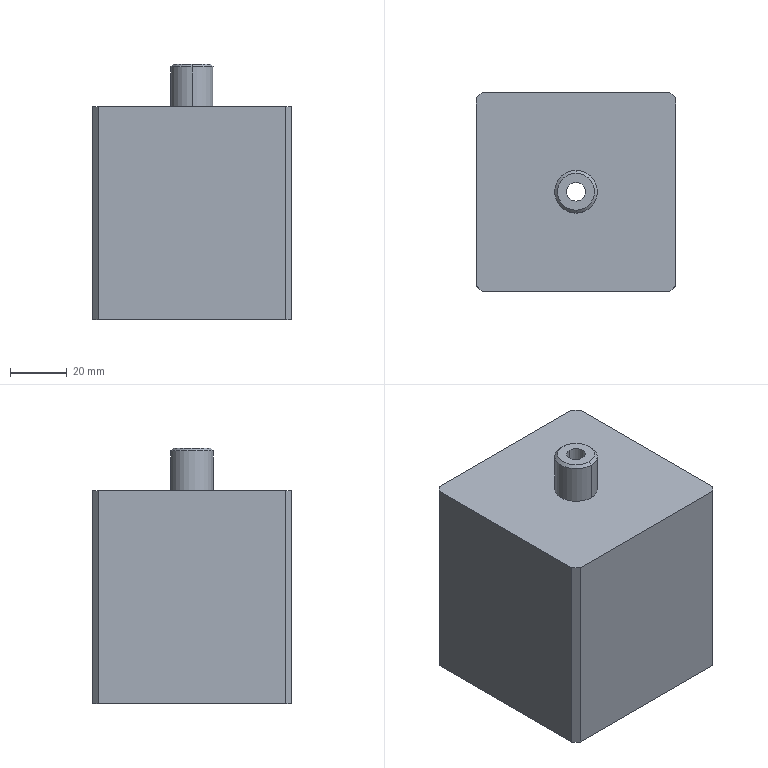Part | NX | 2 solids | 32 faces | box 70 x 70 x 90 mm | volume 242635 mm3 | plane 15 | cylinder 11 | cone 4 | torus 2 | commonest cylinder face diameters 6.6 x4 61.281 x3 4 x2 15 x2
STEP:
#1=CARTESIAN_POINT('',(0.,3.3,0.));
#2=VERTEX_POINT('',#1);
#3=CARTESIAN_POINT('',(0.,-3.3,0.));
#4=VERTEX_POINT('',#3);
#5=CARTESIAN_POINT('',(0.,0.,0.));
#6=DIRECTION('',(0.,0.,-1.));
#7=DIRECTION('',(0.,-1.,0.));
#8=AXIS2_PLACEMENT_3D('',#5,#6,#7);
#9=CIRCLE('',#8,3.3);
#10=EDGE_CURVE('',#2,#4,#9,.T.);
#11=ORIENTED_EDGE('',*,*,#10,.F.);
#12=CARTESIAN_POINT('',(0.,3.3,-15.));
#13=VERTEX_POINT('',#12);
#14=CARTESIAN_POINT('',(0.,3.3,-22.));
#15=DIRECTION('',(0.,0.,-1.));
#16=VECTOR('',#15,1000.);
#17=LINE('',#14,#16);
#18=EDGE_CURVE('',#13,#2,#17,.F.);
#19=ORIENTED_EDGE('',*,*,#18,.F.);
#20=CARTESIAN_POINT('',(0.,-3.3,-15.));
#21=VERTEX_POINT('',#20);
#22=CARTESIAN_POINT('',(0.,0.,-15.));
#23=DIRECTION('',(0.,0.,1.));
#24=DIRECTION('',(0.,1.,0.));
#25=AXIS2_PLACEMENT_3D('',#22,#23,#24);
#26=CIRCLE('',#25,3.3);
#27=EDGE_CURVE('',#21,#13,#26,.T.);
#28=ORIENTED_EDGE('',*,*,#27,.F.);
#29=CARTESIAN_POINT('',(0.,-3.3,-22.));
#30=DIRECTION('',(0.,0.,-1.));
#31=VECTOR('',#30,1000.);
#32=LINE('',#29,#31);
#33=EDGE_CURVE('',#21,#4,#32,.F.);
#34=ORIENTED_EDGE('',*,*,#33,.T.);
#35=EDGE_LOOP('',(#11,#19,#28,#34));
#36=FACE_BOUND('',#35,.T.);
#37=CARTESIAN_POINT('',(0.,0.,-22.));
#38=DIRECTION('',(0.,0.,-1.));
#39=DIRECTION('',(0.,1.,0.));
#40=AXIS2_PLACEMENT_3D('',#37,#38,#39);
#41=CYLINDRICAL_SURFACE('',#40,3.3);
#42=ADVANCED_FACE('',(#36),#41,.F.);
#43=CARTESIAN_POINT('',(0.,6.5,0.));
#44=VERTEX_POINT('',#43);
#45=CARTESIAN_POINT('',(0.,-6.5,0.));
#46=VERTEX_POINT('',#45);
#47=CARTESIAN_POINT('',(0.,0.,0.));
#48=DIRECTION('',(0.,0.,1.));
#49=DIRECTION('',(0.,1.,0.));
#50=AXIS2_PLACEMENT_3D('',#47,#48,#49);
#51=CIRCLE('',#50,6.5);
#52=EDGE_CURVE('',#44,#46,#51,.T.);
#53=ORIENTED_EDGE('',*,*,#52,.F.);
#54=CARTESIAN_POINT('',(0.,7.5,-1.));
#55=VERTEX_POINT('',#54);
#56=CARTESIAN_POINT('',(0.,6.5,0.));
#57=DIRECTION('',(0.,0.7071,-0.7071));
#58=VECTOR('',#57,1000.);
#59=LINE('',#56,#58);
#60=EDGE_CURVE('',#55,#44,#59,.F.);
#61=ORIENTED_EDGE('',*,*,#60,.F.);
#62=CARTESIAN_POINT('',(0.,-7.5,-1.));
#63=VERTEX_POINT('',#62);
#64=CARTESIAN_POINT('',(0.,0.,-1.));
#65=DIRECTION('',(0.,0.,-1.));
#66=DIRECTION('',(0.,1.,0.));
#67=AXIS2_PLACEMENT_3D('',#64,#65,#66);
#68=CIRCLE('',#67,7.5);
#69=EDGE_CURVE('',#63,#55,#68,.T.);
#70=ORIENTED_EDGE('',*,*,#69,.F.);
#71=CARTESIAN_POINT('',(0.,-6.5,0.));
#72=DIRECTION('',(0.,-0.7071,-0.7071));
#73=VECTOR('',#72,1000.);
#74=LINE('',#71,#73);
#75=EDGE_CURVE('',#63,#46,#74,.F.);
#76=ORIENTED_EDGE('',*,*,#75,.T.);
#77=EDGE_LOOP('',(#53,#61,#70,#76));
#78=FACE_BOUND('',#77,.T.);
#79=CARTESIAN_POINT('',(0.,0.,0.));
#80=DIRECTION('',(0.,0.,-1.));
#81=DIRECTION('',(0.,1.,0.));
#82=AXIS2_PLACEMENT_3D('',#79,#80,#81);
#83=CONICAL_SURFACE('',#82,6.5,0.7854);
#84=ADVANCED_FACE('',(#78),#83,.T.);
#85=ORIENTED_EDGE('',*,*,#69,.T.);
#86=CARTESIAN_POINT('',(0.,7.5,-15.));
#87=VERTEX_POINT('',#86);
#88=CARTESIAN_POINT('',(0.,7.5,0.));
#89=DIRECTION('',(0.,0.,-1.));
#90=VECTOR('',#89,1000.);
#91=LINE('',#88,#90);
#92=EDGE_CURVE('',#87,#55,#91,.F.);
#93=ORIENTED_EDGE('',*,*,#92,.F.);
#94=CARTESIAN_POINT('',(0.,-7.5,-15.));
#95=VERTEX_POINT('',#94);
#96=CARTESIAN_POINT('',(0.,0.,-15.));
#97=DIRECTION('',(0.,0.,1.));
#98=DIRECTION('',(0.,1.,0.));
#99=AXIS2_PLACEMENT_3D('',#96,#97,#98);
#100=CIRCLE('',#99,7.5);
#101=EDGE_CURVE('',#87,#95,#100,.T.);
#102=ORIENTED_EDGE('',*,*,#101,.T.);
#103=CARTESIAN_POINT('',(0.,-7.5,0.));
#104=DIRECTION('',(0.,0.,-1.));
#105=VECTOR('',#104,1000.);
#106=LINE('',#103,#105);
#107=EDGE_CURVE('',#95,#63,#106,.F.);
#108=ORIENTED_EDGE('',*,*,#107,.T.);
#109=EDGE_LOOP('',(#85,#93,#102,#108));
#110=FACE_BOUND('',#109,.T.);
#111=CARTESIAN_POINT('',(0.,0.,0.));
#112=DIRECTION('',(0.,0.,-1.));
#113=DIRECTION('',(0.,1.,0.));
#114=AXIS2_PLACEMENT_3D('',#111,#112,#113);
#115=CYLINDRICAL_SURFACE('',#114,7.5);
#116=ADVANCED_FACE('',(#110),#115,.T.);
#117=ORIENTED_EDGE('',*,*,#92,.T.);
#118=CARTESIAN_POINT('',(0.,0.,-1.));
#119=DIRECTION('',(0.,0.,-1.));
#120=DIRECTION('',(0.,1.,0.));
#121=AXIS2_PLACEMENT_3D('',#118,#119,#120);
#122=CIRCLE('',#121,7.5);
#123=EDGE_CURVE('',#55,#63,#122,.T.);
#124=ORIENTED_EDGE('',*,*,#123,.T.);
#125=ORIENTED_EDGE('',*,*,#107,.F.);
#126=CARTESIAN_POINT('',(0.,0.,-15.));
#127=DIRECTION('',(0.,0.,1.));
#128=DIRECTION('',(0.,1.,0.));
#129=AXIS2_PLACEMENT_3D('',#126,#127,#128);
#130=CIRCLE('',#129,7.5);
#131=EDGE_CURVE('',#95,#87,#130,.T.);
#132=ORIENTED_EDGE('',*,*,#131,.T.);
#133=EDGE_LOOP('',(#117,#124,#125,#132));
#134=FACE_BOUND('',#133,.T.);
#135=CARTESIAN_POINT('',(0.,0.,0.));
#136=DIRECTION('',(0.,0.,-1.));
#137=DIRECTION('',(0.,1.,0.));
#138=AXIS2_PLACEMENT_3D('',#135,#136,#137);
#139=CYLINDRICAL_SURFACE('',#138,7.5);
#140=ADVANCED_FACE('',(#134),#139,.T.);
#141=CARTESIAN_POINT('',(0.,0.,0.));
#142=DIRECTION('',(0.,0.,-1.));
#143=DIRECTION('',(0.,-1.,0.));
#144=AXIS2_PLACEMENT_3D('',#141,#142,#143);
#145=CIRCLE('',#144,3.3);
#146=EDGE_CURVE('',#4,#2,#145,.T.);
#147=ORIENTED_EDGE('',*,*,#146,.T.);
#148=ORIENTED_EDGE('',*,*,#10,.T.);
#149=EDGE_LOOP('',(#147,#148));
#150=FACE_BOUND('',#149,.T.);
#151=CARTESIAN_POINT('',(0.,0.,0.));
#152=DIRECTION('',(0.,0.,1.));
#153=DIRECTION('',(0.,1.,0.));
#154=AXIS2_PLACEMENT_3D('',#151,#152,#153);
#155=CIRCLE('',#154,6.5);
#156=EDGE_CURVE('',#46,#44,#155,.T.);
#157=ORIENTED_EDGE('',*,*,#156,.T.);
#158=ORIENTED_EDGE('',*,*,#52,.T.);
#159=EDGE_LOOP('',(#157,#158));
#160=FACE_BOUND('',#159,.T.);
#161=CARTESIAN_POINT('',(0.,0.,0.));
#162=DIRECTION('',(0.,0.,1.));
#163=DIRECTION('',(0.,-1.,0.));
#164=AXIS2_PLACEMENT_3D('',#161,#162,#163);
#165=PLANE('',#164);
#166=ADVANCED_FACE('',(#150,#160),#165,.T.);
#167=ORIENTED_EDGE('',*,*,#27,.T.);
#168=CARTESIAN_POINT('',(0.,0.,-15.));
#169=DIRECTION('',(0.,0.,1.));
#170=DIRECTION('',(0.,1.,0.));
#171=AXIS2_PLACEMENT_3D('',#168,#169,#170);
#172=CIRCLE('',#171,3.3);
#173=EDGE_CURVE('',#13,#21,#172,.T.);
#174=ORIENTED_EDGE('',*,*,#173,.T.);
#175=EDGE_LOOP('',(#167,#174));
#176=FACE_BOUND('',#175,.T.);
#177=ORIENTED_EDGE('',*,*,#131,.F.);
#178=ORIENTED_EDGE('',*,*,#101,.F.);
#179=EDGE_LOOP('',(#177,#178));
#180=FACE_BOUND('',#179,.T.);
#181=CARTESIAN_POINT('',(0.,0.,-15.));
#182=DIRECTION('',(0.,0.,1.));
#183=DIRECTION('',(0.,-1.,0.));
#184=AXIS2_PLACEMENT_3D('',#181,#182,#183);
#185=PLANE('',#184);
#186=ADVANCED_FACE('',(#176,#180),#185,.F.);
#187=ORIENTED_EDGE('',*,*,#60,.T.);
#188=ORIENTED_EDGE('',*,*,#156,.F.);
#189=ORIENTED_EDGE('',*,*,#75,.F.);
#190=ORIENTED_EDGE('',*,*,#123,.F.);
#191=EDGE_LOOP('',(#187,#188,#189,#190));
#192=FACE_BOUND('',#191,.T.);
#193=CARTESIAN_POINT('',(0.,0.,0.));
#194=DIRECTION('',(0.,0.,-1.));
#195=DIRECTION('',(0.,1.,0.));
#196=AXIS2_PLACEMENT_3D('',#193,#194,#195);
#197=CONICAL_SURFACE('',#196,6.5,0.7854);
#198=ADVANCED_FACE('',(#192),#197,.T.);
#199=ORIENTED_EDGE('',*,*,#18,.T.);
#200=ORIENTED_EDGE('',*,*,#146,.F.);
#201=ORIENTED_EDGE('',*,*,#33,.F.);
#202=ORIENTED_EDGE('',*,*,#173,.F.);
#203=EDGE_LOOP('',(#199,#200,#201,#202));
#204=FACE_BOUND('',#203,.T.);
#205=CARTESIAN_POINT('',(0.,0.,-22.));
#206=DIRECTION('',(0.,0.,-1.));
#207=DIRECTION('',(0.,1.,0.));
#208=AXIS2_PLACEMENT_3D('',#205,#206,#207);
#209=CYLINDRICAL_SURFACE('',#208,3.3);
#210=ADVANCED_FACE('',(#204),#209,.F.);
#211=CLOSED_SHELL('',(#42,#84,#116,#140,#166,#186,#198,#210));
#212=MANIFOLD_SOLID_BREP('',#211);
#213=CARTESIAN_POINT('',(0.,3.3,-18.9));
#214=VERTEX_POINT('',#213);
#215=CARTESIAN_POINT('',(0.,-3.3,-18.9));
#216=VERTEX_POINT('',#215);
#217=CARTESIAN_POINT('',(0.,0.,-18.9));
#218=DIRECTION('',(0.,0.,-1.));
#219=DIRECTION('',(0.,-1.,0.));
#220=AXIS2_PLACEMENT_3D('',#217,#218,#219);
#221=CIRCLE('',#220,3.3);
#222=EDGE_CURVE('',#214,#216,#221,.T.);
#223=ORIENTED_EDGE('',*,*,#222,.F.);
#224=CARTESIAN_POINT('',(0.,6.4,-22.));
#225=VERTEX_POINT('',#224);
#226=CARTESIAN_POINT('',(0.,6.4,-22.));
#227=DIRECTION('',(0.,0.7071,-0.7071));
#228=VECTOR('',#227,1000.);
#229=LINE('',#226,#228);
#230=EDGE_CURVE('',#225,#214,#229,.F.);
#231=ORIENTED_EDGE('',*,*,#230,.F.);
#232=CARTESIAN_POINT('',(0.,-6.4,-22.));
#233=VERTEX_POINT('',#232);
#234=CARTESIAN_POINT('',(0.,0.,-22.));
#235=DIRECTION('',(0.,0.,-1.));
#236=DIRECTION('',(0.,-1.,0.));
#237=AXIS2_PLACEMENT_3D('',#234,#235,#236);
#238=CIRCLE('',#237,6.4);
#239=EDGE_CURVE('',#225,#233,#238,.T.);
#240=ORIENTED_EDGE('',*,*,#239,.T.);
#241=CARTESIAN_POINT('',(0.,-6.4,-22.));
#242=DIRECTION('',(0.,-0.7071,-0.7071));
#243=VECTOR('',#242,1000.);
#244=LINE('',#241,#243);
#245=EDGE_CURVE('',#233,#216,#244,.F.);
#246=ORIENTED_EDGE('',*,*,#245,.T.);
#247=EDGE_LOOP('',(#223,#231,#240,#246));
#248=FACE_BOUND('',#247,.T.);
#249=CARTESIAN_POINT('',(0.,0.,-22.));
#250=DIRECTION('',(0.,0.,-1.));
#251=DIRECTION('',(0.,1.,0.));
#252=AXIS2_PLACEMENT_3D('',#249,#250,#251);
#253=CONICAL_SURFACE('',#252,6.4,0.7854);
#254=ADVANCED_FACE('',(#248),#253,.F.);
#255=CARTESIAN_POINT('',(0.,-3.3,-15.));
#256=VERTEX_POINT('',#255);
#257=CARTESIAN_POINT('',(0.,3.3,-15.));
#258=VERTEX_POINT('',#257);
#259=CARTESIAN_POINT('',(0.,0.,-15.));
#260=DIRECTION('',(0.,0.,1.));
#261=DIRECTION('',(0.,1.,0.));
#262=AXIS2_PLACEMENT_3D('',#259,#260,#261);
#263=CIRCLE('',#262,3.3);
#264=EDGE_CURVE('',#256,#258,#263,.T.);
#265=ORIENTED_EDGE('',*,*,#264,.T.);
#266=CARTESIAN_POINT('',(0.,3.3,-22.));
#267=DIRECTION('',(0.,0.,-1.));
#268=VECTOR('',#267,1000.);
#269=LINE('',#266,#268);
#270=EDGE_CURVE('',#214,#258,#269,.F.);
#271=ORIENTED_EDGE('',*,*,#270,.F.);
#272=ORIENTED_EDGE('',*,*,#222,.T.);
#273=CARTESIAN_POINT('',(0.,-3.3,-22.));
#274=DIRECTION('',(0.,0.,-1.));
#275=VECTOR('',#274,1000.);
#276=LINE('',#273,#275);
#277=EDGE_CURVE('',#216,#256,#276,.F.);
#278=ORIENTED_EDGE('',*,*,#277,.T.);
#279=EDGE_LOOP('',(#265,#271,#272,#278));
#280=FACE_BOUND('',#279,.T.);
#281=CARTESIAN_POINT('',(0.,0.,-22.));
#282=DIRECTION('',(0.,0.,-1.));
#283=DIRECTION('',(0.,1.,0.));
#284=AXIS2_PLACEMENT_3D('',#281,#282,#283);
#285=CYLINDRICAL_SURFACE('',#284,3.3);
#286=ADVANCED_FACE('',(#280),#285,.F.);
#287=CARTESIAN_POINT('',(0.,-23.2,-22.));
#288=VERTEX_POINT('',#287);
#289=CARTESIAN_POINT('',(0.,-23.2,-88.));
#290=VERTEX_POINT('',#289);
#291=CARTESIAN_POINT('',(0.,-23.2,-22.));
#292=DIRECTION('',(0.,0.,-1.));
#293=VECTOR('',#292,1000.);
#294=LINE('',#291,#293);
#295=EDGE_CURVE('',#288,#290,#294,.T.);
#296=ORIENTED_EDGE('',*,*,#295,.T.);
#297=CARTESIAN_POINT('',(-23.2,-12.574,-88.));
#298=VERTEX_POINT('',#297);
#299=CARTESIAN_POINT('',(0.,7.44,-88.));
#300=DIRECTION('',(0.,0.,1.));
#301=DIRECTION('',(1.,0.,0.));
#302=AXIS2_PLACEMENT_3D('',#299,#300,#301);
#303=CIRCLE('',#302,30.64);
#304=EDGE_CURVE('',#290,#298,#303,.F.);
#305=ORIENTED_EDGE('',*,*,#304,.T.);
#306=CARTESIAN_POINT('',(-23.2,-12.574,-22.));
#307=VERTEX_POINT('',#306);
#308=CARTESIAN_POINT('',(-23.2,-12.574,-22.));
#309=DIRECTION('',(0.,0.,-1.));
#310=VECTOR('',#309,1000.);
#311=LINE('',#308,#310);
#312=EDGE_CURVE('',#307,#298,#311,.T.);
#313=ORIENTED_EDGE('',*,*,#312,.F.);
#314=CARTESIAN_POINT('',(0.,7.44,-22.));
#315=DIRECTION('',(0.,0.,1.));
#316=DIRECTION('',(1.,0.,0.));
#317=AXIS2_PLACEMENT_3D('',#314,#315,#316);
#318=CIRCLE('',#317,30.64);
#319=EDGE_CURVE('',#288,#307,#318,.F.);
#320=ORIENTED_EDGE('',*,*,#319,.F.);
#321=EDGE_LOOP('',(#296,#305,#313,#320));
#322=FACE_BOUND('',#321,.T.);
#323=CARTESIAN_POINT('',(0.,7.44,-22.));
#324=DIRECTION('',(0.,0.,-1.));
#325=DIRECTION('',(0.,1.,0.));
#326=AXIS2_PLACEMENT_3D('',#323,#324,#325);
#327=CYLINDRICAL_SURFACE('',#326,30.64);
#328=ADVANCED_FACE('',(#322),#327,.F.);
#329=CARTESIAN_POINT('',(-25.2,-13.305,-90.));
#330=VERTEX_POINT('',#329);
#331=CARTESIAN_POINT('',(25.2,-13.305,-90.));
#332=VERTEX_POINT('',#331);
#333=CARTESIAN_POINT('',(0.,7.44,-90.));
#334=DIRECTION('',(0.,0.,1.));
#335=DIRECTION('',(1.,0.,0.));
#336=AXIS2_PLACEMENT_3D('',#333,#334,#335);
#337=CIRCLE('',#336,32.64);
#338=EDGE_CURVE('',#330,#332,#337,.T.);
#339=ORIENTED_EDGE('',*,*,#338,.T.);
#340=CARTESIAN_POINT('',(25.2,13.305,-90.));
#341=VERTEX_POINT('',#340);
#342=CARTESIAN_POINT('',(25.2,12.574,-90.));
#343=DIRECTION('',(0.,1.,0.));
#344=VECTOR('',#343,1000.);
#345=LINE('',#342,#344);
#346=EDGE_CURVE('',#332,#341,#345,.T.);
#347=ORIENTED_EDGE('',*,*,#346,.T.);
#348=CARTESIAN_POINT('',(-25.2,13.305,-90.));
#349=VERTEX_POINT('',#348);
#350=CARTESIAN_POINT('',(0.,-7.44,-90.));
#351=DIRECTION('',(0.,0.,1.));
#352=DIRECTION('',(1.,0.,0.));
#353=AXIS2_PLACEMENT_3D('',#350,#351,#352);
#354=CIRCLE('',#353,32.64);
#355=EDGE_CURVE('',#341,#349,#354,.T.);
#356=ORIENTED_EDGE('',*,*,#355,.T.);
#357=CARTESIAN_POINT('',(-25.2,0.,-90.));
#358=DIRECTION('',(0.,-1.,0.));
#359=VECTOR('',#358,1000.);
#360=LINE('',#357,#359);
#361=EDGE_CURVE('',#349,#330,#360,.T.);
#362=ORIENTED_EDGE('',*,*,#361,.T.);
#363=EDGE_LOOP('',(#339,#347,#356,#362));
#364=FACE_BOUND('',#363,.T.);
#365=CARTESIAN_POINT('',(33.,35.,-90.));
#366=VERTEX_POINT('',#365);
#367=CARTESIAN_POINT('',(-33.,35.,-90.));
#368=VERTEX_POINT('',#367);
#369=CARTESIAN_POINT('',(35.,35.,-90.));
#370=DIRECTION('',(-1.,0.,0.));
#371=VECTOR('',#370,1000.);
#372=LINE('',#369,#371);
#373=EDGE_CURVE('',#366,#368,#372,.T.);
#374=ORIENTED_EDGE('',*,*,#373,.F.);
#375=CARTESIAN_POINT('',(35.,33.,-90.));
#376=VERTEX_POINT('',#375);
#377=CARTESIAN_POINT('',(35.,33.,-90.));
#378=DIRECTION('',(0.7071,-0.7071,0.));
#379=VECTOR('',#378,1000.);
#380=LINE('',#377,#379);
#381=EDGE_CURVE('',#366,#376,#380,.T.);
#382=ORIENTED_EDGE('',*,*,#381,.T.);
#383=CARTESIAN_POINT('',(35.,-33.,-90.));
#384=VERTEX_POINT('',#383);
#385=CARTESIAN_POINT('',(35.,-35.,-90.));
#386=DIRECTION('',(0.,1.,0.));
#387=VECTOR('',#386,1000.);
#388=LINE('',#385,#387);
#389=EDGE_CURVE('',#384,#376,#388,.T.);
#390=ORIENTED_EDGE('',*,*,#389,.F.);
#391=CARTESIAN_POINT('',(33.,-35.,-90.));
#392=VERTEX_POINT('',#391);
#393=CARTESIAN_POINT('',(33.,-35.,-90.));
#394=DIRECTION('',(-0.7071,-0.7071,0.));
#395=VECTOR('',#394,1000.);
#396=LINE('',#393,#395);
#397=EDGE_CURVE('',#384,#392,#396,.T.);
#398=ORIENTED_EDGE('',*,*,#397,.T.);
#399=CARTESIAN_POINT('',(-33.,-35.,-90.));
#400=VERTEX_POINT('',#399);
#401=CARTESIAN_POINT('',(35.,-35.,-90.));
#402=DIRECTION('',(-1.,0.,0.));
#403=VECTOR('',#402,1000.);
#404=LINE('',#401,#403);
#405=EDGE_CURVE('',#392,#400,#404,.T.);
#406=ORIENTED_EDGE('',*,*,#405,.T.);
#407=CARTESIAN_POINT('',(-35.,-33.,-90.));
#408=VERTEX_POINT('',#407);
#409=CARTESIAN_POINT('',(-35.,-33.,-90.));
#410=DIRECTION('',(-0.7071,0.7071,0.));
#411=VECTOR('',#410,1000.);
#412=LINE('',#409,#411);
#413=EDGE_CURVE('',#400,#408,#412,.T.);
#414=ORIENTED_EDGE('',*,*,#413,.T.);
#415=CARTESIAN_POINT('',(-35.,33.,-90.));
#416=VERTEX_POINT('',#415);
#417=CARTESIAN_POINT('',(-35.,-35.,-90.));
#418=DIRECTION('',(0.,1.,0.));
#419=VECTOR('',#418,1000.);
#420=LINE('',#417,#419);
#421=EDGE_CURVE('',#408,#416,#420,.T.);
#422=ORIENTED_EDGE('',*,*,#421,.T.);
#423=CARTESIAN_POINT('',(-33.,35.,-90.));
#424=DIRECTION('',(0.7071,0.7071,0.));
#425=VECTOR('',#424,1000.);
#426=LINE('',#423,#425);
#427=EDGE_CURVE('',#416,#368,#426,.T.);
#428=ORIENTED_EDGE('',*,*,#427,.T.);
#429=EDGE_LOOP('',(#374,#382,#390,#398,#406,#414,#422,#428));
#430=FACE_BOUND('',#429,.T.);
#431=CARTESIAN_POINT('',(0.,0.,-90.));
#432=DIRECTION('',(0.,0.,1.));
#433=DIRECTION('',(0.,-1.,0.));
#434=AXIS2_PLACEMENT_3D('',#431,#432,#433);
#435=PLANE('',#434);
#436=ADVANCED_FACE('',(#364,#430),#435,.F.);
#437=ORIENTED_EDGE('',*,*,#389,.T.);
#438=CARTESIAN_POINT('',(35.,33.,-15.));
#439=VERTEX_POINT('',#438);
#440=CARTESIAN_POINT('',(35.,33.,-90.));
#441=DIRECTION('',(0.,0.,1.));
#442=VECTOR('',#441,1000.);
#443=LINE('',#440,#442);
#444=EDGE_CURVE('',#376,#439,#443,.T.);
#445=ORIENTED_EDGE('',*,*,#444,.T.);
#446=CARTESIAN_POINT('',(35.,-33.,-15.));
#447=VERTEX_POINT('',#446);
#448=CARTESIAN_POINT('',(35.,-35.,-15.));
#449=DIRECTION('',(0.,1.,0.));
#450=VECTOR('',#449,1000.);
#451=LINE('',#448,#450);
#452=EDGE_CURVE('',#447,#439,#451,.T.);
#453=ORIENTED_EDGE('',*,*,#452,.F.);
#454=CARTESIAN_POINT('',(35.,-33.,-90.));
#455=DIRECTION('',(0.,0.,-1.));
#456=VECTOR('',#455,1000.);
#457=LINE('',#454,#456);
#458=EDGE_CURVE('',#447,#384,#457,.T.);
#459=ORIENTED_EDGE('',*,*,#458,.T.);
#460=EDGE_LOOP('',(#437,#445,#453,#459));
#461=FACE_BOUND('',#460,.T.);
#462=CARTESIAN_POINT('',(35.,-35.,-90.));
#463=DIRECTION('',(1.,0.,0.));
#464=DIRECTION('',(0.,1.,0.));
#465=AXIS2_PLACEMENT_3D('',#462,#463,#464);
#466=PLANE('',#465);
#467=ADVANCED_FACE('',(#461),#466,.T.);
#468=ORIENTED_EDGE('',*,*,#405,.F.);
#469=CARTESIAN_POINT('',(33.,-35.,-15.));
#470=VERTEX_POINT('',#469);
#471=CARTESIAN_POINT('',(33.,-35.,-15.));
#472=DIRECTION('',(0.,0.,1.));
#473=VECTOR('',#472,1000.);
#474=LINE('',#471,#473);
#475=EDGE_CURVE('',#392,#470,#474,.T.);
#476=ORIENTED_EDGE('',*,*,#475,.T.);
#477=CARTESIAN_POINT('',(-33.,-35.,-15.));
#478=VERTEX_POINT('',#477);
#479=CARTESIAN_POINT('',(35.,-35.,-15.));
#480=DIRECTION('',(-1.,0.,0.));
#481=VECTOR('',#480,1000.);
#482=LINE('',#479,#481);
#483=EDGE_CURVE('',#470,#478,#482,.T.);
#484=ORIENTED_EDGE('',*,*,#483,.T.);
#485=CARTESIAN_POINT('',(-33.,-35.,-90.));
#486=DIRECTION('',(0.,0.,-1.));
#487=VECTOR('',#486,1000.);
#488=LINE('',#485,#487);
#489=EDGE_CURVE('',#478,#400,#488,.T.);
#490=ORIENTED_EDGE('',*,*,#489,.T.);
#491=EDGE_LOOP('',(#468,#476,#484,#490));
#492=FACE_BOUND('',#491,.T.);
#493=CARTESIAN_POINT('',(35.,-35.,-90.));
#494=DIRECTION('',(0.,1.,0.));
#495=DIRECTION('',(-1.,0.,0.));
#496=AXIS2_PLACEMENT_3D('',#493,#494,#495);
#497=PLANE('',#496);
#498=ADVANCED_FACE('',(#492),#497,.F.);
#499=ORIENTED_EDGE('',*,*,#421,.F.);
#500=CARTESIAN_POINT('',(-35.,-33.,-15.));
#501=VERTEX_POINT('',#500);
#502=CARTESIAN_POINT('',(-35.,-33.,-90.));
#503=DIRECTION('',(0.,0.,1.));
#504=VECTOR('',#503,1000.);
#505=LINE('',#502,#504);
#506=EDGE_CURVE('',#408,#501,#505,.T.);
#507=ORIENTED_EDGE('',*,*,#506,.T.);
#508=CARTESIAN_POINT('',(-35.,33.,-15.));
#509=VERTEX_POINT('',#508);
#510=CARTESIAN_POINT('',(-35.,-35.,-15.));
#511=DIRECTION('',(0.,1.,0.));
#512=VECTOR('',#511,1000.);
#513=LINE('',#510,#512);
#514=EDGE_CURVE('',#501,#509,#513,.T.);
#515=ORIENTED_EDGE('',*,*,#514,.T.);
#516=CARTESIAN_POINT('',(-35.,33.,-90.));
#517=DIRECTION('',(0.,0.,-1.));
#518=VECTOR('',#517,1000.);
#519=LINE('',#516,#518);
#520=EDGE_CURVE('',#509,#416,#519,.T.);
#521=ORIENTED_EDGE('',*,*,#520,.T.);
#522=EDGE_LOOP('',(#499,#507,#515,#521));
#523=FACE_BOUND('',#522,.T.);
#524=CARTESIAN_POINT('',(-35.,-35.,-90.));
#525=DIRECTION('',(1.,0.,0.));
#526=DIRECTION('',(0.,1.,0.));
#527=AXIS2_PLACEMENT_3D('',#524,#525,#526);
#528=PLANE('',#527);
#529=ADVANCED_FACE('',(#523),#528,.F.);
#530=CARTESIAN_POINT('',(33.,35.,-15.));
#531=VERTEX_POINT('',#530);
#532=CARTESIAN_POINT('',(-33.,35.,-15.));
#533=VERTEX_POINT('',#532);
#534=CARTESIAN_POINT('',(35.,35.,-15.));
#535=DIRECTION('',(-1.,0.,0.));
#536=VECTOR('',#535,1000.);
#537=LINE('',#534,#536);
#538=EDGE_CURVE('',#531,#533,#537,.T.);
#539=ORIENTED_EDGE('',*,*,#538,.F.);
#540=CARTESIAN_POINT('',(33.,35.,-90.));
#541=DIRECTION('',(0.,0.,-1.));
#542=VECTOR('',#541,1000.);
#543=LINE('',#540,#542);
#544=EDGE_CURVE('',#531,#366,#543,.T.);
#545=ORIENTED_EDGE('',*,*,#544,.T.);
#546=ORIENTED_EDGE('',*,*,#373,.T.);
#547=CARTESIAN_POINT('',(-33.,35.,-15.));
#548=DIRECTION('',(0.,0.,1.));
#549=VECTOR('',#548,1000.);
#550=LINE('',#547,#549);
#551=EDGE_CURVE('',#368,#533,#550,.T.);
#552=ORIENTED_EDGE('',*,*,#551,.T.);
#553=EDGE_LOOP('',(#539,#545,#546,#552));
#554=FACE_BOUND('',#553,.T.);
#555=CARTESIAN_POINT('',(35.,35.,-90.));
#556=DIRECTION('',(0.,1.,0.));
#557=DIRECTION('',(-1.,0.,0.));
#558=AXIS2_PLACEMENT_3D('',#555,#556,#557);
#559=PLANE('',#558);
#560=ADVANCED_FACE('',(#554),#559,.T.);
#561=ORIENTED_EDGE('',*,*,#264,.F.);
#562=CARTESIAN_POINT('',(0.,0.,-15.));
#563=DIRECTION('',(0.,0.,1.));
#564=DIRECTION('',(0.,1.,0.));
#565=AXIS2_PLACEMENT_3D('',#562,#563,#564);
#566=CIRCLE('',#565,3.3);
#567=EDGE_CURVE('',#258,#256,#566,.T.);
#568=ORIENTED_EDGE('',*,*,#567,.F.);
#569=EDGE_LOOP('',(#561,#568));
#570=FACE_BOUND('',#569,.T.);
#571=ORIENTED_EDGE('',*,*,#452,.T.);
#572=CARTESIAN_POINT('',(34.,34.,-15.));
#573=DIRECTION('',(-0.7071,0.7071,0.));
#574=VECTOR('',#573,1000.);
#575=LINE('',#572,#574);
#576=EDGE_CURVE('',#439,#531,#575,.T.);
#577=ORIENTED_EDGE('',*,*,#576,.T.);
#578=ORIENTED_EDGE('',*,*,#538,.T.);
#579=CARTESIAN_POINT('',(-34.,34.,-15.));
#580=DIRECTION('',(-0.7071,-0.7071,0.));
#581=VECTOR('',#580,1000.);
#582=LINE('',#579,#581);
#583=EDGE_CURVE('',#533,#509,#582,.T.);
#584=ORIENTED_EDGE('',*,*,#583,.T.);
#585=ORIENTED_EDGE('',*,*,#514,.F.);
#586=CARTESIAN_POINT('',(-34.,-34.,-15.));
#587=DIRECTION('',(0.7071,-0.7071,0.));
#588=VECTOR('',#587,1000.);
#589=LINE('',#586,#588);
#590=EDGE_CURVE('',#501,#478,#589,.T.);
#591=ORIENTED_EDGE('',*,*,#590,.T.);
#592=ORIENTED_EDGE('',*,*,#483,.F.);
#593=CARTESIAN_POINT('',(34.,-34.,-15.));
#594=DIRECTION('',(0.7071,0.7071,0.));
#595=VECTOR('',#594,1000.);
#596=LINE('',#593,#595);
#597=EDGE_CURVE('',#470,#447,#596,.T.);
#598=ORIENTED_EDGE('',*,*,#597,.T.);
#599=EDGE_LOOP('',(#571,#577,#578,#584,#585,#591,#592,#598));
#600=FACE_BOUND('',#599,.T.);
#601=CARTESIAN_POINT('',(0.,0.,-15.));
#602=DIRECTION('',(0.,0.,1.));
#603=DIRECTION('',(0.,-1.,0.));
#604=AXIS2_PLACEMENT_3D('',#601,#602,#603);
#605=PLANE('',#604);
#606=ADVANCED_FACE('',(#570,#600),#605,.T.);
#607=CARTESIAN_POINT('',(23.2,12.574,-22.));
#608=VERTEX_POINT('',#607);
#609=CARTESIAN_POINT('',(23.2,12.574,-88.));
#610=VERTEX_POINT('',#609);
#611=CARTESIAN_POINT('',(23.2,12.574,-22.));
#612=DIRECTION('',(0.,0.,-1.));
#613=VECTOR('',#612,1000.);
#614=LINE('',#611,#613);
#615=EDGE_CURVE('',#608,#610,#614,.T.);
#616=ORIENTED_EDGE('',*,*,#615,.T.);
#617=CARTESIAN_POINT('',(23.2,-12.574,-88.));
#618=VERTEX_POINT('',#617);
#619=CARTESIAN_POINT('',(23.2,-12.574,-88.));
#620=DIRECTION('',(0.,1.,0.));
#621=VECTOR('',#620,1000.);
#622=LINE('',#619,#621);
#623=EDGE_CURVE('',#610,#618,#622,.F.);
#624=ORIENTED_EDGE('',*,*,#623,.T.);
#625=CARTESIAN_POINT('',(23.2,-12.574,-22.));
#626=VERTEX_POINT('',#625);
#627=CARTESIAN_POINT('',(23.2,-12.574,-22.));
#628=DIRECTION('',(0.,0.,-1.));
#629=VECTOR('',#628,1000.);
#630=LINE('',#627,#629);
#631=EDGE_CURVE('',#626,#618,#630,.T.);
#632=ORIENTED_EDGE('',*,*,#631,.F.);
#633=CARTESIAN_POINT('',(23.2,-12.5,-22.));
#634=DIRECTION('',(0.,1.,0.));
#635=VECTOR('',#634,1000.);
#636=LINE('',#633,#635);
#637=EDGE_CURVE('',#626,#608,#636,.T.);
#638=ORIENTED_EDGE('',*,*,#637,.T.);
#639=EDGE_LOOP('',(#616,#624,#632,#638));
#640=FACE_BOUND('',#639,.T.);
#641=CARTESIAN_POINT('',(23.2,-12.5,-22.));
#642=DIRECTION('',(-1.,0.,0.));
#643=DIRECTION('',(0.,-1.,0.));
#644=AXIS2_PLACEMENT_3D('',#641,#642,#643);
#645=PLANE('',#644);
#646=ADVANCED_FACE('',(#640),#645,.T.);
#647=CARTESIAN_POINT('',(-23.2,12.574,-22.));
#648=VERTEX_POINT('',#647);
#649=CARTESIAN_POINT('',(-23.2,12.574,-88.));
#650=VERTEX_POINT('',#649);
#651=CARTESIAN_POINT('',(-23.2,12.574,-22.));
#652=DIRECTION('',(0.,0.,-1.));
#653=VECTOR('',#652,1000.);
#654=LINE('',#651,#653);
#655=EDGE_CURVE('',#648,#650,#654,.T.);
#656=ORIENTED_EDGE('',*,*,#655,.T.);
#657=CARTESIAN_POINT('',(0.,-7.44,-88.));
#658=DIRECTION('',(0.,0.,1.));
#659=DIRECTION('',(1.,0.,0.));
#660=AXIS2_PLACEMENT_3D('',#657,#658,#659);
#661=CIRCLE('',#660,30.64);
#662=EDGE_CURVE('',#650,#610,#661,.F.);
#663=ORIENTED_EDGE('',*,*,#662,.T.);
#664=ORIENTED_EDGE('',*,*,#615,.F.);
#665=CARTESIAN_POINT('',(0.,-7.44,-22.));
#666=DIRECTION('',(0.,0.,1.));
#667=DIRECTION('',(1.,0.,0.));
#668=AXIS2_PLACEMENT_3D('',#665,#666,#667);
#669=CIRCLE('',#668,30.64);
#670=EDGE_CURVE('',#608,#648,#669,.T.);
#671=ORIENTED_EDGE('',*,*,#670,.T.);
#672=EDGE_LOOP('',(#656,#663,#664,#671));
#673=FACE_BOUND('',#672,.T.);
#674=CARTESIAN_POINT('',(0.,-7.44,-22.));
#675=DIRECTION('',(0.,0.,-1.));
#676=DIRECTION('',(0.,1.,0.));
#677=AXIS2_PLACEMENT_3D('',#674,#675,#676);
#678=CYLINDRICAL_SURFACE('',#677,30.64);
#679=ADVANCED_FACE('',(#673),#678,.F.);
#680=ORIENTED_EDGE('',*,*,#312,.T.);
#681=CARTESIAN_POINT('',(-23.2,-12.5,-88.));
#682=DIRECTION('',(0.,-1.,0.));
#683=VECTOR('',#682,1000.);
#684=LINE('',#681,#683);
#685=EDGE_CURVE('',#298,#650,#684,.F.);
#686=ORIENTED_EDGE('',*,*,#685,.T.);
#687=ORIENTED_EDGE('',*,*,#655,.F.);
#688=CARTESIAN_POINT('',(-23.2,-12.5,-22.));
#689=DIRECTION('',(0.,1.,0.));
#690=VECTOR('',#689,1000.);
#691=LINE('',#688,#690);
#692=EDGE_CURVE('',#307,#648,#691,.T.);
#693=ORIENTED_EDGE('',*,*,#692,.F.);
#694=EDGE_LOOP('',(#680,#686,#687,#693));
#695=FACE_BOUND('',#694,.T.);
#696=CARTESIAN_POINT('',(-23.2,-12.5,-22.));
#697=DIRECTION('',(-1.,0.,0.));
#698=DIRECTION('',(0.,-1.,0.));
#699=AXIS2_PLACEMENT_3D('',#696,#697,#698);
#700=PLANE('',#699);
#701=ADVANCED_FACE('',(#695),#700,.F.);
#702=ORIENTED_EDGE('',*,*,#631,.T.);
#703=CARTESIAN_POINT('',(0.,7.44,-88.));
#704=DIRECTION('',(0.,0.,1.));
#705=DIRECTION('',(1.,0.,0.));
#706=AXIS2_PLACEMENT_3D('',#703,#704,#705);
#707=CIRCLE('',#706,30.64);
#708=EDGE_CURVE('',#618,#290,#707,.F.);
#709=ORIENTED_EDGE('',*,*,#708,.T.);
#710=ORIENTED_EDGE('',*,*,#295,.F.);
#711=CARTESIAN_POINT('',(0.,7.44,-22.));
#712=DIRECTION('',(0.,0.,1.));
#713=DIRECTION('',(1.,0.,0.));
#714=AXIS2_PLACEMENT_3D('',#711,#712,#713);
#715=CIRCLE('',#714,30.64);
#716=EDGE_CURVE('',#626,#288,#715,.F.);
#717=ORIENTED_EDGE('',*,*,#716,.F.);
#718=EDGE_LOOP('',(#702,#709,#710,#717));
#719=FACE_BOUND('',#718,.T.);
#720=CARTESIAN_POINT('',(0.,7.44,-22.));
#721=DIRECTION('',(0.,0.,-1.));
#722=DIRECTION('',(0.,1.,0.));
#723=AXIS2_PLACEMENT_3D('',#720,#721,#722);
#724=CYLINDRICAL_SURFACE('',#723,30.64);
#725=ADVANCED_FACE('',(#719),#724,.F.);
#726=CARTESIAN_POINT('',(0.,0.,-22.));
#727=DIRECTION('',(0.,0.,-1.));
#728=DIRECTION('',(0.,-1.,0.));
#729=AXIS2_PLACEMENT_3D('',#726,#727,#728);
#730=CIRCLE('',#729,6.4);
#731=EDGE_CURVE('',#233,#225,#730,.T.);
#732=ORIENTED_EDGE('',*,*,#731,.F.);
#733=ORIENTED_EDGE('',*,*,#239,.F.);
#734=EDGE_LOOP('',(#732,#733));
#735=FACE_BOUND('',#734,.T.);
#736=ORIENTED_EDGE('',*,*,#637,.F.);
#737=ORIENTED_EDGE('',*,*,#716,.T.);
#738=ORIENTED_EDGE('',*,*,#319,.T.);
#739=ORIENTED_EDGE('',*,*,#692,.T.);
#740=ORIENTED_EDGE('',*,*,#670,.F.);
#741=EDGE_LOOP('',(#736,#737,#738,#739,#740));
#742=FACE_BOUND('',#741,.T.);
#743=CARTESIAN_POINT('',(0.,-7.44,-22.));
#744=DIRECTION('',(0.,0.,1.));
#745=DIRECTION('',(0.,-1.,0.));
#746=AXIS2_PLACEMENT_3D('',#743,#744,#745);
#747=PLANE('',#746);
#748=ADVANCED_FACE('',(#735,#742),#747,.F.);
#749=ORIENTED_EDGE('',*,*,#381,.F.);
#750=ORIENTED_EDGE('',*,*,#544,.F.);
#751=ORIENTED_EDGE('',*,*,#576,.F.);
#752=ORIENTED_EDGE('',*,*,#444,.F.);
#753=EDGE_LOOP('',(#749,#750,#751,#752));
#754=FACE_BOUND('',#753,.T.);
#755=CARTESIAN_POINT('',(35.,33.,-90.));
#756=DIRECTION('',(-0.7071,-0.7071,0.));
#757=DIRECTION('',(0.,0.,-1.));
#758=AXIS2_PLACEMENT_3D('',#755,#756,#757);
#759=PLANE('',#758);
#760=ADVANCED_FACE('',(#754),#759,.F.);
#761=ORIENTED_EDGE('',*,*,#397,.F.);
#762=ORIENTED_EDGE('',*,*,#458,.F.);
#763=ORIENTED_EDGE('',*,*,#597,.F.);
#764=ORIENTED_EDGE('',*,*,#475,.F.);
#765=EDGE_LOOP('',(#761,#762,#763,#764));
#766=FACE_BOUND('',#765,.T.);
#767=CARTESIAN_POINT('',(33.,-35.,-90.));
#768=DIRECTION('',(0.7071,-0.7071,0.));
#769=DIRECTION('',(0.,0.,1.));
#770=AXIS2_PLACEMENT_3D('',#767,#768,#769);
#771=PLANE('',#770);
#772=ADVANCED_FACE('',(#766),#771,.T.);
#773=ORIENTED_EDGE('',*,*,#413,.F.);
#774=ORIENTED_EDGE('',*,*,#489,.F.);
#775=ORIENTED_EDGE('',*,*,#590,.F.);
#776=ORIENTED_EDGE('',*,*,#506,.F.);
#777=EDGE_LOOP('',(#773,#774,#775,#776));
#778=FACE_BOUND('',#777,.T.);
#779=CARTESIAN_POINT('',(-35.,-33.,-90.));
#780=DIRECTION('',(0.7071,0.7071,0.));
#781=DIRECTION('',(0.,0.,-1.));
#782=AXIS2_PLACEMENT_3D('',#779,#780,#781);
#783=PLANE('',#782);
#784=ADVANCED_FACE('',(#778),#783,.F.);
#785=ORIENTED_EDGE('',*,*,#427,.F.);
#786=ORIENTED_EDGE('',*,*,#520,.F.);
#787=ORIENTED_EDGE('',*,*,#583,.F.);
#788=ORIENTED_EDGE('',*,*,#551,.F.);
#789=EDGE_LOOP('',(#785,#786,#787,#788));
#790=FACE_BOUND('',#789,.T.);
#791=CARTESIAN_POINT('',(-33.,35.,-90.));
#792=DIRECTION('',(-0.7071,0.7071,0.));
#793=DIRECTION('',(0.,0.,1.));
#794=AXIS2_PLACEMENT_3D('',#791,#792,#793);
#795=PLANE('',#794);
#796=ADVANCED_FACE('',(#790),#795,.T.);
#797=ORIENTED_EDGE('',*,*,#270,.T.);
#798=ORIENTED_EDGE('',*,*,#567,.T.);
#799=ORIENTED_EDGE('',*,*,#277,.F.);
#800=CARTESIAN_POINT('',(0.,0.,-18.9));
#801=DIRECTION('',(0.,0.,-1.));
#802=DIRECTION('',(0.,-1.,0.));
#803=AXIS2_PLACEMENT_3D('',#800,#801,#802);
#804=CIRCLE('',#803,3.3);
#805=EDGE_CURVE('',#216,#214,#804,.T.);
#806=ORIENTED_EDGE('',*,*,#805,.T.);
#807=EDGE_LOOP('',(#797,#798,#799,#806));
#808=FACE_BOUND('',#807,.T.);
#809=CARTESIAN_POINT('',(0.,0.,-22.));
#810=DIRECTION('',(0.,0.,-1.));
#811=DIRECTION('',(0.,1.,0.));
#812=AXIS2_PLACEMENT_3D('',#809,#810,#811);
#813=CYLINDRICAL_SURFACE('',#812,3.3);
#814=ADVANCED_FACE('',(#808),#813,.F.);
#815=ORIENTED_EDGE('',*,*,#230,.T.);
#816=ORIENTED_EDGE('',*,*,#805,.F.);
#817=ORIENTED_EDGE('',*,*,#245,.F.);
#818=ORIENTED_EDGE('',*,*,#731,.T.);
#819=EDGE_LOOP('',(#815,#816,#817,#818));
#820=FACE_BOUND('',#819,.T.);
#821=CARTESIAN_POINT('',(0.,0.,-22.));
#822=DIRECTION('',(0.,0.,-1.));
#823=DIRECTION('',(0.,1.,0.));
#824=AXIS2_PLACEMENT_3D('',#821,#822,#823);
#825=CONICAL_SURFACE('',#824,6.4,0.7854);
#826=ADVANCED_FACE('',(#820),#825,.F.);
#827=ORIENTED_EDGE('',*,*,#304,.F.);
#828=ORIENTED_EDGE('',*,*,#708,.F.);
#829=CARTESIAN_POINT('',(23.2,-12.574,-88.));
#830=CARTESIAN_POINT('',(23.2,-12.574,-88.546));
#831=CARTESIAN_POINT('',(23.667,-12.749,-89.598));
#832=CARTESIAN_POINT('',(24.694,-13.123,-90.));
#833=CARTESIAN_POINT('',(25.2,-13.305,-90.));
#834=B_SPLINE_CURVE_WITH_KNOTS('',3,(#829,#830,#831,#832,#833),.UNSPECIFIED.,.F.,.F.,(4,1,4),(0.,0.001613,0.003226),.UNSPECIFIED.);
#835=EDGE_CURVE('',#332,#618,#834,.F.);
#836=ORIENTED_EDGE('',*,*,#835,.F.);
#837=ORIENTED_EDGE('',*,*,#338,.F.);
#838=CARTESIAN_POINT('',(-23.2,-12.574,-88.));
#839=CARTESIAN_POINT('',(-23.2,-12.574,-88.546));
#840=CARTESIAN_POINT('',(-23.667,-12.749,-89.598));
#841=CARTESIAN_POINT('',(-24.694,-13.123,-90.));
#842=CARTESIAN_POINT('',(-25.2,-13.305,-90.));
#843=B_SPLINE_CURVE_WITH_KNOTS('',3,(#838,#839,#840,#841,#842),.UNSPECIFIED.,.F.,.F.,(4,1,4),(0.,0.001613,0.003226),.UNSPECIFIED.);
#844=EDGE_CURVE('',#298,#330,#843,.T.);
#845=ORIENTED_EDGE('',*,*,#844,.F.);
#846=EDGE_LOOP('',(#827,#828,#836,#837,#845));
#847=FACE_BOUND('',#846,.T.);
#848=CARTESIAN_POINT('',(0.,7.44,-88.));
#849=DIRECTION('',(0.,0.,1.));
#850=DIRECTION('',(1.,0.,0.));
#851=AXIS2_PLACEMENT_3D('',#848,#849,#850);
#852=TOROIDAL_SURFACE('',#851,32.64,2.);
#853=ADVANCED_FACE('',(#847),#852,.T.);
#854=ORIENTED_EDGE('',*,*,#844,.T.);
#855=ORIENTED_EDGE('',*,*,#361,.F.);
#856=CARTESIAN_POINT('',(-23.2,12.574,-88.));
#857=CARTESIAN_POINT('',(-23.2,12.574,-88.546));
#858=CARTESIAN_POINT('',(-23.667,12.749,-89.598));
#859=CARTESIAN_POINT('',(-24.694,13.123,-90.));
#860=CARTESIAN_POINT('',(-25.2,13.305,-90.));
#861=B_SPLINE_CURVE_WITH_KNOTS('',3,(#856,#857,#858,#859,#860),.UNSPECIFIED.,.F.,.F.,(4,1,4),(0.,0.001613,0.003226),.UNSPECIFIED.);
#862=EDGE_CURVE('',#650,#349,#861,.T.);
#863=ORIENTED_EDGE('',*,*,#862,.F.);
#864=ORIENTED_EDGE('',*,*,#685,.F.);
#865=EDGE_LOOP('',(#854,#855,#863,#864));
#866=FACE_BOUND('',#865,.T.);
#867=CARTESIAN_POINT('',(-25.2,0.,-88.));
#868=DIRECTION('',(0.,-1.,0.));
#869=DIRECTION('',(0.,0.,-1.));
#870=AXIS2_PLACEMENT_3D('',#867,#868,#869);
#871=CYLINDRICAL_SURFACE('',#870,2.);
#872=ADVANCED_FACE('',(#866),#871,.T.);
#873=ORIENTED_EDGE('',*,*,#862,.T.);
#874=ORIENTED_EDGE('',*,*,#355,.F.);
#875=CARTESIAN_POINT('',(23.2,12.574,-88.));
#876=CARTESIAN_POINT('',(23.2,12.574,-88.546));
#877=CARTESIAN_POINT('',(23.667,12.749,-89.598));
#878=CARTESIAN_POINT('',(24.694,13.123,-90.));
#879=CARTESIAN_POINT('',(25.2,13.305,-90.));
#880=B_SPLINE_CURVE_WITH_KNOTS('',3,(#875,#876,#877,#878,#879),.UNSPECIFIED.,.F.,.F.,(4,1,4),(0.,0.001613,0.003226),.UNSPECIFIED.);
#881=EDGE_CURVE('',#610,#341,#880,.T.);
#882=ORIENTED_EDGE('',*,*,#881,.F.);
#883=ORIENTED_EDGE('',*,*,#662,.F.);
#884=EDGE_LOOP('',(#873,#874,#882,#883));
#885=FACE_BOUND('',#884,.T.);
#886=CARTESIAN_POINT('',(0.,-7.44,-88.));
#887=DIRECTION('',(0.,0.,1.));
#888=DIRECTION('',(1.,0.,0.));
#889=AXIS2_PLACEMENT_3D('',#886,#887,#888);
#890=TOROIDAL_SURFACE('',#889,32.64,2.);
#891=ADVANCED_FACE('',(#885),#890,.T.);
#892=ORIENTED_EDGE('',*,*,#835,.T.);
#893=ORIENTED_EDGE('',*,*,#623,.F.);
#894=ORIENTED_EDGE('',*,*,#881,.T.);
#895=ORIENTED_EDGE('',*,*,#346,.F.);
#896=EDGE_LOOP('',(#892,#893,#894,#895));
#897=FACE_BOUND('',#896,.T.);
#898=CARTESIAN_POINT('',(25.2,0.,-88.));
#899=DIRECTION('',(0.,-1.,0.));
#900=DIRECTION('',(0.,0.,-1.));
#901=AXIS2_PLACEMENT_3D('',#898,#899,#900);
#902=CYLINDRICAL_SURFACE('',#901,2.);
#903=ADVANCED_FACE('',(#897),#902,.T.);
#904=CLOSED_SHELL('',(#254,#286,#328,#436,#467,#498,#529,#560,#606,#646,#679,#701,#725,#748,#760,#772,#784,#796,#814,#826,#853,#872,#891,#903));
#905=MANIFOLD_SOLID_BREP('',#904);
#906=(LENGTH_UNIT()NAMED_UNIT(*)SI_UNIT(.MILLI.,.METRE.));
#907=UNCERTAINTY_MEASURE_WITH_UNIT(LENGTH_MEASURE(0.0508),#906,'','');
#908=(NAMED_UNIT(*)PLANE_ANGLE_UNIT()SI_UNIT($,.RADIAN.));
#909=(NAMED_UNIT(*)SI_UNIT($,.STERADIAN.)SOLID_ANGLE_UNIT());
#910=(GEOMETRIC_REPRESENTATION_CONTEXT(3)GLOBAL_UNCERTAINTY_ASSIGNED_CONTEXT((#907))GLOBAL_UNIT_ASSIGNED_CONTEXT((#906,#908,#909))REPRESENTATION_CONTEXT('',''));
#911=ADVANCED_BREP_SHAPE_REPRESENTATION('',(#212,#905),#910);